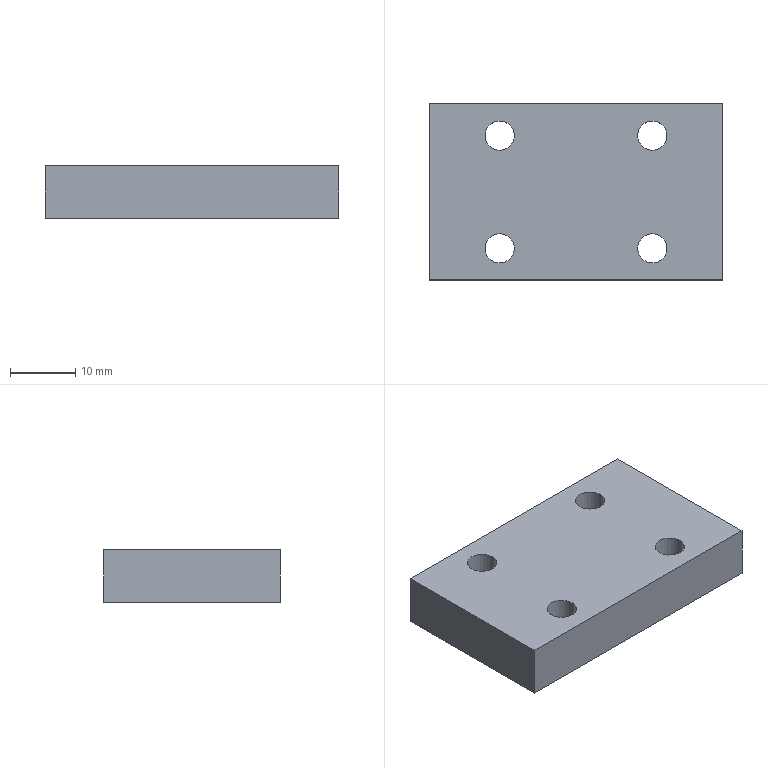Part | SolidWorks | features BaseBody 1 | 1 solid | 14 faces | box 45 x 27 x 8 mm | volume 9211 mm3 | cylinder 8 | plane 6 | commonest cylinder face diameters 4.5 x8
STEP:
#1=CARTESIAN_POINT('',(9.45,8.64,28.));
#2=VERTEX_POINT('',#1);
#3=CARTESIAN_POINT('',(13.95,8.64,28.));
#4=VERTEX_POINT('',#3);
#5=CARTESIAN_POINT('',(11.7,8.64,28.));
#6=DIRECTION('',(0.,0.,1.));
#7=DIRECTION('',(1.,0.,0.));
#8=AXIS2_PLACEMENT_3D('',#5,#6,#7);
#9=CIRCLE('',#8,2.25);
#10=EDGE_CURVE('',#2,#4,#9,.T.);
#11=ORIENTED_EDGE('',*,*,#10,.F.);
#12=CARTESIAN_POINT('',(9.45,8.64,36.));
#13=VERTEX_POINT('',#12);
#14=CARTESIAN_POINT('',(9.45,8.64,27.));
#15=DIRECTION('',(0.,0.,1.));
#16=VECTOR('',#15,1000.);
#17=LINE('',#14,#16);
#18=EDGE_CURVE('',#2,#13,#17,.T.);
#19=ORIENTED_EDGE('',*,*,#18,.T.);
#20=CARTESIAN_POINT('',(13.95,8.64,36.));
#21=VERTEX_POINT('',#20);
#22=CARTESIAN_POINT('',(11.7,8.64,36.));
#23=DIRECTION('',(0.,0.,-1.));
#24=DIRECTION('',(1.,0.,0.));
#25=AXIS2_PLACEMENT_3D('',#22,#23,#24);
#26=CIRCLE('',#25,2.25);
#27=EDGE_CURVE('',#21,#13,#26,.T.);
#28=ORIENTED_EDGE('',*,*,#27,.F.);
#29=CARTESIAN_POINT('',(13.95,8.64,27.));
#30=DIRECTION('',(0.,0.,1.));
#31=VECTOR('',#30,1000.);
#32=LINE('',#29,#31);
#33=EDGE_CURVE('',#4,#21,#32,.T.);
#34=ORIENTED_EDGE('',*,*,#33,.F.);
#35=EDGE_LOOP('',(#11,#19,#28,#34));
#36=FACE_OUTER_BOUND('',#35,.T.);
#37=CARTESIAN_POINT('',(11.7,8.64,27.));
#38=DIRECTION('',(0.,0.,1.));
#39=DIRECTION('',(1.,0.,0.));
#40=AXIS2_PLACEMENT_3D('',#37,#38,#39);
#41=CYLINDRICAL_SURFACE('',#40,2.25);
#42=ADVANCED_FACE('',(#36),#41,.F.);
#43=CARTESIAN_POINT('',(-13.95,8.64,28.));
#44=VERTEX_POINT('',#43);
#45=CARTESIAN_POINT('',(-9.45,8.64,28.));
#46=VERTEX_POINT('',#45);
#47=CARTESIAN_POINT('',(-11.7,8.64,28.));
#48=DIRECTION('',(0.,0.,1.));
#49=DIRECTION('',(1.,0.,0.));
#50=AXIS2_PLACEMENT_3D('',#47,#48,#49);
#51=CIRCLE('',#50,2.25);
#52=EDGE_CURVE('',#44,#46,#51,.T.);
#53=ORIENTED_EDGE('',*,*,#52,.F.);
#54=CARTESIAN_POINT('',(-13.95,8.64,36.));
#55=VERTEX_POINT('',#54);
#56=CARTESIAN_POINT('',(-13.95,8.64,27.));
#57=DIRECTION('',(0.,0.,1.));
#58=VECTOR('',#57,1000.);
#59=LINE('',#56,#58);
#60=EDGE_CURVE('',#44,#55,#59,.T.);
#61=ORIENTED_EDGE('',*,*,#60,.T.);
#62=CARTESIAN_POINT('',(-9.45,8.64,36.));
#63=VERTEX_POINT('',#62);
#64=CARTESIAN_POINT('',(-11.7,8.64,36.));
#65=DIRECTION('',(0.,0.,-1.));
#66=DIRECTION('',(1.,0.,0.));
#67=AXIS2_PLACEMENT_3D('',#64,#65,#66);
#68=CIRCLE('',#67,2.25);
#69=EDGE_CURVE('',#63,#55,#68,.T.);
#70=ORIENTED_EDGE('',*,*,#69,.F.);
#71=CARTESIAN_POINT('',(-9.45,8.64,27.));
#72=DIRECTION('',(0.,0.,1.));
#73=VECTOR('',#72,1000.);
#74=LINE('',#71,#73);
#75=EDGE_CURVE('',#46,#63,#74,.T.);
#76=ORIENTED_EDGE('',*,*,#75,.F.);
#77=EDGE_LOOP('',(#53,#61,#70,#76));
#78=FACE_OUTER_BOUND('',#77,.T.);
#79=CARTESIAN_POINT('',(-11.7,8.64,27.));
#80=DIRECTION('',(0.,0.,1.));
#81=DIRECTION('',(1.,0.,0.));
#82=AXIS2_PLACEMENT_3D('',#79,#80,#81);
#83=CYLINDRICAL_SURFACE('',#82,2.25);
#84=ADVANCED_FACE('',(#78),#83,.F.);
#85=CARTESIAN_POINT('',(9.45,-8.64,28.));
#86=VERTEX_POINT('',#85);
#87=CARTESIAN_POINT('',(13.95,-8.64,28.));
#88=VERTEX_POINT('',#87);
#89=CARTESIAN_POINT('',(11.7,-8.64,28.));
#90=DIRECTION('',(0.,0.,1.));
#91=DIRECTION('',(1.,0.,0.));
#92=AXIS2_PLACEMENT_3D('',#89,#90,#91);
#93=CIRCLE('',#92,2.25);
#94=EDGE_CURVE('',#86,#88,#93,.T.);
#95=ORIENTED_EDGE('',*,*,#94,.F.);
#96=CARTESIAN_POINT('',(9.45,-8.64,36.));
#97=VERTEX_POINT('',#96);
#98=CARTESIAN_POINT('',(9.45,-8.64,27.));
#99=DIRECTION('',(0.,0.,1.));
#100=VECTOR('',#99,1000.);
#101=LINE('',#98,#100);
#102=EDGE_CURVE('',#86,#97,#101,.T.);
#103=ORIENTED_EDGE('',*,*,#102,.T.);
#104=CARTESIAN_POINT('',(13.95,-8.64,36.));
#105=VERTEX_POINT('',#104);
#106=CARTESIAN_POINT('',(11.7,-8.64,36.));
#107=DIRECTION('',(0.,0.,-1.));
#108=DIRECTION('',(1.,0.,0.));
#109=AXIS2_PLACEMENT_3D('',#106,#107,#108);
#110=CIRCLE('',#109,2.25);
#111=EDGE_CURVE('',#105,#97,#110,.T.);
#112=ORIENTED_EDGE('',*,*,#111,.F.);
#113=CARTESIAN_POINT('',(13.95,-8.64,27.));
#114=DIRECTION('',(0.,0.,1.));
#115=VECTOR('',#114,1000.);
#116=LINE('',#113,#115);
#117=EDGE_CURVE('',#88,#105,#116,.T.);
#118=ORIENTED_EDGE('',*,*,#117,.F.);
#119=EDGE_LOOP('',(#95,#103,#112,#118));
#120=FACE_OUTER_BOUND('',#119,.T.);
#121=CARTESIAN_POINT('',(11.7,-8.64,27.));
#122=DIRECTION('',(0.,0.,1.));
#123=DIRECTION('',(1.,0.,0.));
#124=AXIS2_PLACEMENT_3D('',#121,#122,#123);
#125=CYLINDRICAL_SURFACE('',#124,2.25);
#126=ADVANCED_FACE('',(#120),#125,.F.);
#127=CARTESIAN_POINT('',(-13.95,-8.64,28.));
#128=VERTEX_POINT('',#127);
#129=CARTESIAN_POINT('',(-9.45,-8.64,28.));
#130=VERTEX_POINT('',#129);
#131=CARTESIAN_POINT('',(-11.7,-8.64,28.));
#132=DIRECTION('',(0.,0.,1.));
#133=DIRECTION('',(1.,0.,0.));
#134=AXIS2_PLACEMENT_3D('',#131,#132,#133);
#135=CIRCLE('',#134,2.25);
#136=EDGE_CURVE('',#128,#130,#135,.T.);
#137=ORIENTED_EDGE('',*,*,#136,.F.);
#138=CARTESIAN_POINT('',(-13.95,-8.64,36.));
#139=VERTEX_POINT('',#138);
#140=CARTESIAN_POINT('',(-13.95,-8.64,27.));
#141=DIRECTION('',(0.,0.,1.));
#142=VECTOR('',#141,1000.);
#143=LINE('',#140,#142);
#144=EDGE_CURVE('',#128,#139,#143,.T.);
#145=ORIENTED_EDGE('',*,*,#144,.T.);
#146=CARTESIAN_POINT('',(-9.45,-8.64,36.));
#147=VERTEX_POINT('',#146);
#148=CARTESIAN_POINT('',(-11.7,-8.64,36.));
#149=DIRECTION('',(0.,0.,-1.));
#150=DIRECTION('',(1.,0.,0.));
#151=AXIS2_PLACEMENT_3D('',#148,#149,#150);
#152=CIRCLE('',#151,2.25);
#153=EDGE_CURVE('',#147,#139,#152,.T.);
#154=ORIENTED_EDGE('',*,*,#153,.F.);
#155=CARTESIAN_POINT('',(-9.45,-8.64,27.));
#156=DIRECTION('',(0.,0.,1.));
#157=VECTOR('',#156,1000.);
#158=LINE('',#155,#157);
#159=EDGE_CURVE('',#130,#147,#158,.T.);
#160=ORIENTED_EDGE('',*,*,#159,.F.);
#161=EDGE_LOOP('',(#137,#145,#154,#160));
#162=FACE_OUTER_BOUND('',#161,.T.);
#163=CARTESIAN_POINT('',(-11.7,-8.64,27.));
#164=DIRECTION('',(0.,0.,1.));
#165=DIRECTION('',(1.,0.,0.));
#166=AXIS2_PLACEMENT_3D('',#163,#164,#165);
#167=CYLINDRICAL_SURFACE('',#166,2.25);
#168=ADVANCED_FACE('',(#162),#167,.F.);
#169=ORIENTED_EDGE('',*,*,#27,.T.);
#170=CARTESIAN_POINT('',(11.7,8.64,36.));
#171=DIRECTION('',(0.,0.,-1.));
#172=DIRECTION('',(1.,0.,0.));
#173=AXIS2_PLACEMENT_3D('',#170,#171,#172);
#174=CIRCLE('',#173,2.25);
#175=EDGE_CURVE('',#13,#21,#174,.T.);
#176=ORIENTED_EDGE('',*,*,#175,.T.);
#177=EDGE_LOOP('',(#169,#176));
#178=FACE_BOUND('',#177,.T.);
#179=ORIENTED_EDGE('',*,*,#69,.T.);
#180=CARTESIAN_POINT('',(-11.7,8.64,36.));
#181=DIRECTION('',(0.,0.,-1.));
#182=DIRECTION('',(1.,0.,0.));
#183=AXIS2_PLACEMENT_3D('',#180,#181,#182);
#184=CIRCLE('',#183,2.25);
#185=EDGE_CURVE('',#55,#63,#184,.T.);
#186=ORIENTED_EDGE('',*,*,#185,.T.);
#187=EDGE_LOOP('',(#179,#186));
#188=FACE_BOUND('',#187,.T.);
#189=ORIENTED_EDGE('',*,*,#111,.T.);
#190=CARTESIAN_POINT('',(11.7,-8.64,36.));
#191=DIRECTION('',(0.,0.,-1.));
#192=DIRECTION('',(1.,0.,0.));
#193=AXIS2_PLACEMENT_3D('',#190,#191,#192);
#194=CIRCLE('',#193,2.25);
#195=EDGE_CURVE('',#97,#105,#194,.T.);
#196=ORIENTED_EDGE('',*,*,#195,.T.);
#197=EDGE_LOOP('',(#189,#196));
#198=FACE_BOUND('',#197,.T.);
#199=ORIENTED_EDGE('',*,*,#153,.T.);
#200=CARTESIAN_POINT('',(-11.7,-8.64,36.));
#201=DIRECTION('',(0.,0.,-1.));
#202=DIRECTION('',(1.,0.,0.));
#203=AXIS2_PLACEMENT_3D('',#200,#201,#202);
#204=CIRCLE('',#203,2.25);
#205=EDGE_CURVE('',#139,#147,#204,.T.);
#206=ORIENTED_EDGE('',*,*,#205,.T.);
#207=EDGE_LOOP('',(#199,#206));
#208=FACE_BOUND('',#207,.T.);
#209=CARTESIAN_POINT('',(22.5,-13.5,36.));
#210=VERTEX_POINT('',#209);
#211=CARTESIAN_POINT('',(22.5,13.5,36.));
#212=VERTEX_POINT('',#211);
#213=CARTESIAN_POINT('',(22.5,-13.5,36.));
#214=DIRECTION('',(0.,1.,0.));
#215=VECTOR('',#214,1000.);
#216=LINE('',#213,#215);
#217=EDGE_CURVE('',#210,#212,#216,.T.);
#218=ORIENTED_EDGE('',*,*,#217,.T.);
#219=CARTESIAN_POINT('',(-22.5,13.5,36.));
#220=VERTEX_POINT('',#219);
#221=CARTESIAN_POINT('',(-22.5,13.5,36.));
#222=DIRECTION('',(-1.,0.,0.));
#223=VECTOR('',#222,1000.);
#224=LINE('',#221,#223);
#225=EDGE_CURVE('',#212,#220,#224,.T.);
#226=ORIENTED_EDGE('',*,*,#225,.T.);
#227=CARTESIAN_POINT('',(-22.5,-13.5,36.));
#228=VERTEX_POINT('',#227);
#229=CARTESIAN_POINT('',(-22.5,-13.5,36.));
#230=DIRECTION('',(0.,-1.,0.));
#231=VECTOR('',#230,1000.);
#232=LINE('',#229,#231);
#233=EDGE_CURVE('',#220,#228,#232,.T.);
#234=ORIENTED_EDGE('',*,*,#233,.T.);
#235=CARTESIAN_POINT('',(-22.5,-13.5,36.));
#236=DIRECTION('',(1.,0.,0.));
#237=VECTOR('',#236,1000.);
#238=LINE('',#235,#237);
#239=EDGE_CURVE('',#228,#210,#238,.T.);
#240=ORIENTED_EDGE('',*,*,#239,.T.);
#241=EDGE_LOOP('',(#218,#226,#234,#240));
#242=FACE_OUTER_BOUND('',#241,.T.);
#243=CARTESIAN_POINT('',(-22.5,-13.5,36.));
#244=DIRECTION('',(0.,0.,1.));
#245=DIRECTION('',(1.,0.,0.));
#246=AXIS2_PLACEMENT_3D('',#243,#244,#245);
#247=PLANE('',#246);
#248=ADVANCED_FACE('',(#178,#188,#198,#208,#242),#247,.T.);
#249=ORIENTED_EDGE('',*,*,#18,.F.);
#250=CARTESIAN_POINT('',(11.7,8.64,28.));
#251=DIRECTION('',(0.,0.,1.));
#252=DIRECTION('',(1.,0.,0.));
#253=AXIS2_PLACEMENT_3D('',#250,#251,#252);
#254=CIRCLE('',#253,2.25);
#255=EDGE_CURVE('',#4,#2,#254,.T.);
#256=ORIENTED_EDGE('',*,*,#255,.F.);
#257=ORIENTED_EDGE('',*,*,#33,.T.);
#258=ORIENTED_EDGE('',*,*,#175,.F.);
#259=EDGE_LOOP('',(#249,#256,#257,#258));
#260=FACE_OUTER_BOUND('',#259,.T.);
#261=CARTESIAN_POINT('',(11.7,8.64,27.));
#262=DIRECTION('',(0.,0.,1.));
#263=DIRECTION('',(1.,0.,0.));
#264=AXIS2_PLACEMENT_3D('',#261,#262,#263);
#265=CYLINDRICAL_SURFACE('',#264,2.25);
#266=ADVANCED_FACE('',(#260),#265,.F.);
#267=ORIENTED_EDGE('',*,*,#60,.F.);
#268=CARTESIAN_POINT('',(-11.7,8.64,28.));
#269=DIRECTION('',(0.,0.,1.));
#270=DIRECTION('',(1.,0.,0.));
#271=AXIS2_PLACEMENT_3D('',#268,#269,#270);
#272=CIRCLE('',#271,2.25);
#273=EDGE_CURVE('',#46,#44,#272,.T.);
#274=ORIENTED_EDGE('',*,*,#273,.F.);
#275=ORIENTED_EDGE('',*,*,#75,.T.);
#276=ORIENTED_EDGE('',*,*,#185,.F.);
#277=EDGE_LOOP('',(#267,#274,#275,#276));
#278=FACE_OUTER_BOUND('',#277,.T.);
#279=CARTESIAN_POINT('',(-11.7,8.64,27.));
#280=DIRECTION('',(0.,0.,1.));
#281=DIRECTION('',(1.,0.,0.));
#282=AXIS2_PLACEMENT_3D('',#279,#280,#281);
#283=CYLINDRICAL_SURFACE('',#282,2.25);
#284=ADVANCED_FACE('',(#278),#283,.F.);
#285=ORIENTED_EDGE('',*,*,#102,.F.);
#286=CARTESIAN_POINT('',(11.7,-8.64,28.));
#287=DIRECTION('',(0.,0.,1.));
#288=DIRECTION('',(1.,0.,0.));
#289=AXIS2_PLACEMENT_3D('',#286,#287,#288);
#290=CIRCLE('',#289,2.25);
#291=EDGE_CURVE('',#88,#86,#290,.T.);
#292=ORIENTED_EDGE('',*,*,#291,.F.);
#293=ORIENTED_EDGE('',*,*,#117,.T.);
#294=ORIENTED_EDGE('',*,*,#195,.F.);
#295=EDGE_LOOP('',(#285,#292,#293,#294));
#296=FACE_OUTER_BOUND('',#295,.T.);
#297=CARTESIAN_POINT('',(11.7,-8.64,27.));
#298=DIRECTION('',(0.,0.,1.));
#299=DIRECTION('',(1.,0.,0.));
#300=AXIS2_PLACEMENT_3D('',#297,#298,#299);
#301=CYLINDRICAL_SURFACE('',#300,2.25);
#302=ADVANCED_FACE('',(#296),#301,.F.);
#303=ORIENTED_EDGE('',*,*,#144,.F.);
#304=CARTESIAN_POINT('',(-11.7,-8.64,28.));
#305=DIRECTION('',(0.,0.,1.));
#306=DIRECTION('',(1.,0.,0.));
#307=AXIS2_PLACEMENT_3D('',#304,#305,#306);
#308=CIRCLE('',#307,2.25);
#309=EDGE_CURVE('',#130,#128,#308,.T.);
#310=ORIENTED_EDGE('',*,*,#309,.F.);
#311=ORIENTED_EDGE('',*,*,#159,.T.);
#312=ORIENTED_EDGE('',*,*,#205,.F.);
#313=EDGE_LOOP('',(#303,#310,#311,#312));
#314=FACE_OUTER_BOUND('',#313,.T.);
#315=CARTESIAN_POINT('',(-11.7,-8.64,27.));
#316=DIRECTION('',(0.,0.,1.));
#317=DIRECTION('',(1.,0.,0.));
#318=AXIS2_PLACEMENT_3D('',#315,#316,#317);
#319=CYLINDRICAL_SURFACE('',#318,2.25);
#320=ADVANCED_FACE('',(#314),#319,.F.);
#321=ORIENTED_EDGE('',*,*,#225,.F.);
#322=CARTESIAN_POINT('',(22.5,13.5,28.));
#323=VERTEX_POINT('',#322);
#324=CARTESIAN_POINT('',(22.5,13.5,28.));
#325=DIRECTION('',(0.,0.,-1.));
#326=VECTOR('',#325,1000.);
#327=LINE('',#324,#326);
#328=EDGE_CURVE('',#212,#323,#327,.T.);
#329=ORIENTED_EDGE('',*,*,#328,.T.);
#330=CARTESIAN_POINT('',(-22.5,13.5,28.));
#331=VERTEX_POINT('',#330);
#332=CARTESIAN_POINT('',(-22.5,13.5,28.));
#333=DIRECTION('',(-1.,0.,0.));
#334=VECTOR('',#333,1000.);
#335=LINE('',#332,#334);
#336=EDGE_CURVE('',#323,#331,#335,.T.);
#337=ORIENTED_EDGE('',*,*,#336,.T.);
#338=CARTESIAN_POINT('',(-22.5,13.5,28.));
#339=DIRECTION('',(0.,0.,1.));
#340=VECTOR('',#339,1000.);
#341=LINE('',#338,#340);
#342=EDGE_CURVE('',#331,#220,#341,.T.);
#343=ORIENTED_EDGE('',*,*,#342,.T.);
#344=EDGE_LOOP('',(#321,#329,#337,#343));
#345=FACE_OUTER_BOUND('',#344,.T.);
#346=CARTESIAN_POINT('',(-22.5,13.5,28.));
#347=DIRECTION('',(0.,1.,0.));
#348=DIRECTION('',(0.,0.,1.));
#349=AXIS2_PLACEMENT_3D('',#346,#347,#348);
#350=PLANE('',#349);
#351=ADVANCED_FACE('',(#345),#350,.T.);
#352=ORIENTED_EDGE('',*,*,#328,.F.);
#353=ORIENTED_EDGE('',*,*,#217,.F.);
#354=CARTESIAN_POINT('',(22.5,-13.5,28.));
#355=VERTEX_POINT('',#354);
#356=CARTESIAN_POINT('',(22.5,-13.5,28.));
#357=DIRECTION('',(0.,0.,-1.));
#358=VECTOR('',#357,1000.);
#359=LINE('',#356,#358);
#360=EDGE_CURVE('',#210,#355,#359,.T.);
#361=ORIENTED_EDGE('',*,*,#360,.T.);
#362=CARTESIAN_POINT('',(22.5,-13.5,28.));
#363=DIRECTION('',(0.,1.,0.));
#364=VECTOR('',#363,1000.);
#365=LINE('',#362,#364);
#366=EDGE_CURVE('',#355,#323,#365,.T.);
#367=ORIENTED_EDGE('',*,*,#366,.T.);
#368=EDGE_LOOP('',(#352,#353,#361,#367));
#369=FACE_OUTER_BOUND('',#368,.T.);
#370=CARTESIAN_POINT('',(22.5,-13.5,28.));
#371=DIRECTION('',(1.,0.,0.));
#372=DIRECTION('',(0.,0.,-1.));
#373=AXIS2_PLACEMENT_3D('',#370,#371,#372);
#374=PLANE('',#373);
#375=ADVANCED_FACE('',(#369),#374,.T.);
#376=ORIENTED_EDGE('',*,*,#239,.F.);
#377=CARTESIAN_POINT('',(-22.5,-13.5,28.));
#378=VERTEX_POINT('',#377);
#379=CARTESIAN_POINT('',(-22.5,-13.5,28.));
#380=DIRECTION('',(0.,0.,1.));
#381=VECTOR('',#380,1000.);
#382=LINE('',#379,#381);
#383=EDGE_CURVE('',#378,#228,#382,.T.);
#384=ORIENTED_EDGE('',*,*,#383,.F.);
#385=CARTESIAN_POINT('',(-22.5,-13.5,28.));
#386=DIRECTION('',(-1.,0.,0.));
#387=VECTOR('',#386,1000.);
#388=LINE('',#385,#387);
#389=EDGE_CURVE('',#355,#378,#388,.T.);
#390=ORIENTED_EDGE('',*,*,#389,.F.);
#391=ORIENTED_EDGE('',*,*,#360,.F.);
#392=EDGE_LOOP('',(#376,#384,#390,#391));
#393=FACE_OUTER_BOUND('',#392,.T.);
#394=CARTESIAN_POINT('',(-22.5,-13.5,28.));
#395=DIRECTION('',(0.,1.,0.));
#396=DIRECTION('',(0.,0.,1.));
#397=AXIS2_PLACEMENT_3D('',#394,#395,#396);
#398=PLANE('',#397);
#399=ADVANCED_FACE('',(#393),#398,.F.);
#400=ORIENTED_EDGE('',*,*,#342,.F.);
#401=CARTESIAN_POINT('',(-22.5,-13.5,28.));
#402=DIRECTION('',(0.,1.,0.));
#403=VECTOR('',#402,1000.);
#404=LINE('',#401,#403);
#405=EDGE_CURVE('',#378,#331,#404,.T.);
#406=ORIENTED_EDGE('',*,*,#405,.F.);
#407=ORIENTED_EDGE('',*,*,#383,.T.);
#408=ORIENTED_EDGE('',*,*,#233,.F.);
#409=EDGE_LOOP('',(#400,#406,#407,#408));
#410=FACE_OUTER_BOUND('',#409,.T.);
#411=CARTESIAN_POINT('',(-22.5,-13.5,28.));
#412=DIRECTION('',(1.,0.,0.));
#413=DIRECTION('',(0.,0.,-1.));
#414=AXIS2_PLACEMENT_3D('',#411,#412,#413);
#415=PLANE('',#414);
#416=ADVANCED_FACE('',(#410),#415,.F.);
#417=ORIENTED_EDGE('',*,*,#255,.T.);
#418=ORIENTED_EDGE('',*,*,#10,.T.);
#419=EDGE_LOOP('',(#417,#418));
#420=FACE_BOUND('',#419,.T.);
#421=ORIENTED_EDGE('',*,*,#273,.T.);
#422=ORIENTED_EDGE('',*,*,#52,.T.);
#423=EDGE_LOOP('',(#421,#422));
#424=FACE_BOUND('',#423,.T.);
#425=ORIENTED_EDGE('',*,*,#291,.T.);
#426=ORIENTED_EDGE('',*,*,#94,.T.);
#427=EDGE_LOOP('',(#425,#426));
#428=FACE_BOUND('',#427,.T.);
#429=ORIENTED_EDGE('',*,*,#309,.T.);
#430=ORIENTED_EDGE('',*,*,#136,.T.);
#431=EDGE_LOOP('',(#429,#430));
#432=FACE_BOUND('',#431,.T.);
#433=ORIENTED_EDGE('',*,*,#366,.F.);
#434=ORIENTED_EDGE('',*,*,#389,.T.);
#435=ORIENTED_EDGE('',*,*,#405,.T.);
#436=ORIENTED_EDGE('',*,*,#336,.F.);
#437=EDGE_LOOP('',(#433,#434,#435,#436));
#438=FACE_OUTER_BOUND('',#437,.T.);
#439=CARTESIAN_POINT('',(-22.5,-13.5,28.));
#440=DIRECTION('',(0.,0.,1.));
#441=DIRECTION('',(1.,0.,0.));
#442=AXIS2_PLACEMENT_3D('',#439,#440,#441);
#443=PLANE('',#442);
#444=ADVANCED_FACE('',(#420,#424,#428,#432,#438),#443,.F.);
#445=CLOSED_SHELL('',(#42,#84,#126,#168,#248,#266,#284,#302,#320,#351,#375,#399,#416,#444));
#446=MANIFOLD_SOLID_BREP('',#445);
#447=CARTESIAN_POINT('',(0.,0.,0.));
#448=DIRECTION('',(0.,0.,1.));
#449=DIRECTION('',(1.,0.,0.));
#450=AXIS2_PLACEMENT_3D('',#447,#448,#449);
#451=(LENGTH_UNIT()NAMED_UNIT(*)SI_UNIT(.MILLI.,.METRE.));
#452=UNCERTAINTY_MEASURE_WITH_UNIT(LENGTH_MEASURE(0.00001),#451,'','');
#453=(NAMED_UNIT(*)PLANE_ANGLE_UNIT()SI_UNIT($,.RADIAN.));
#454=(NAMED_UNIT(*)SI_UNIT($,.STERADIAN.)SOLID_ANGLE_UNIT());
#455=(GEOMETRIC_REPRESENTATION_CONTEXT(3)GLOBAL_UNCERTAINTY_ASSIGNED_CONTEXT((#452))GLOBAL_UNIT_ASSIGNED_CONTEXT((#451,#453,#454))REPRESENTATION_CONTEXT('',''));
#456=ADVANCED_BREP_SHAPE_REPRESENTATION('',(#446,#450),#455);